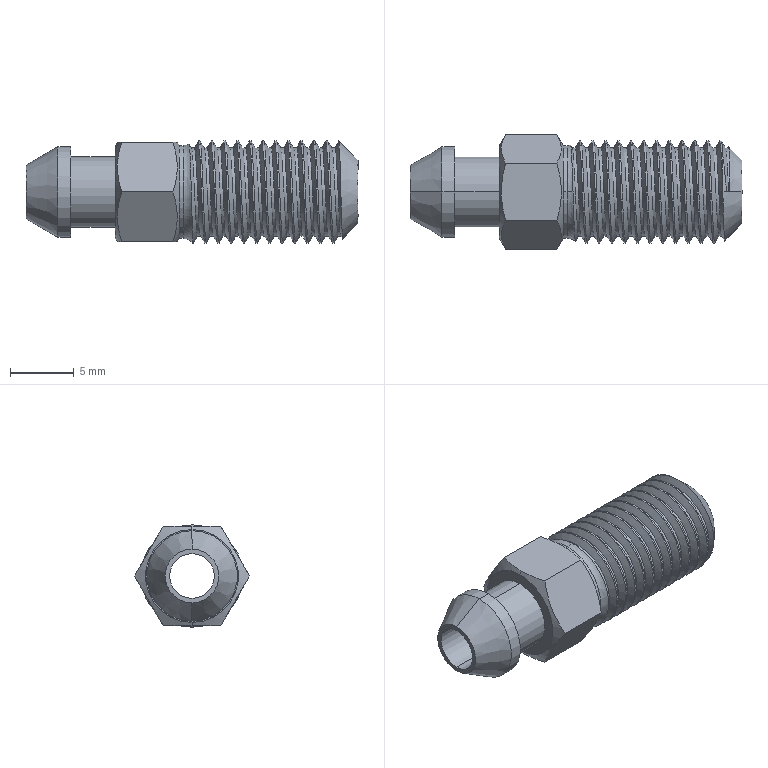Part | SolidWorks | features BaseBody 1 | 1 solid | 59 faces | box 26 x 9.007 x 8 mm | volume 782.255 mm3 | cylinder 32 | plane 12 | cone 9 | spline 3 | torus 3 | commonest cylinder face diameters 8 x24 3.5 x2 5.5 x2 7.1 x2 7.275 x2